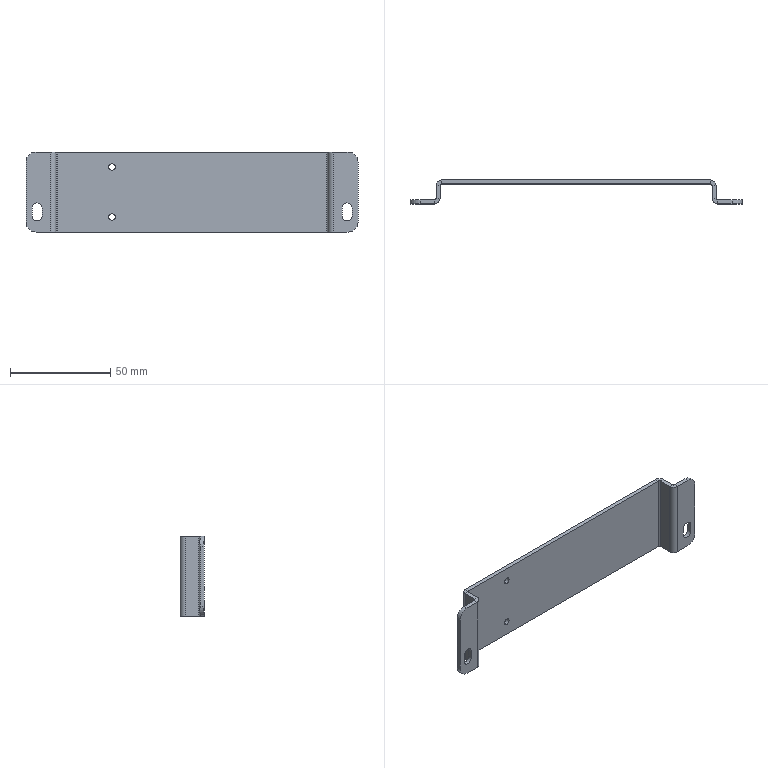Part | STEP file | 1 solid | 56 faces | box 166 x 12 x 40 mm | volume 14406 mm3 | plane 34 | cylinder 22 | commonest cylinder face diameters 5 x6 1.473 x4 3.3 x4 5.473 x4 10 x4